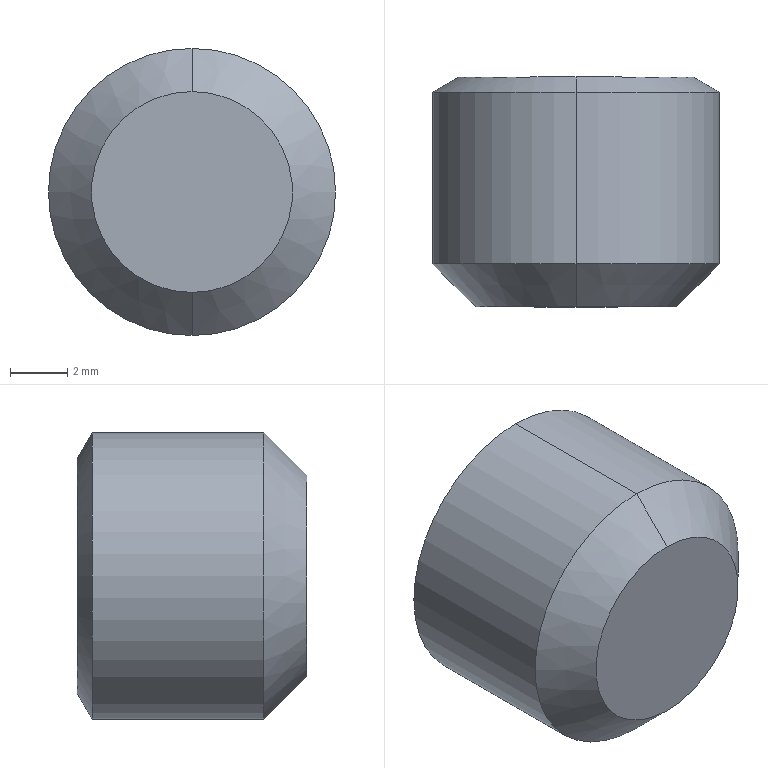Part | STEP file | 0229_Z_SCCN50-22_2 | 1 solid | 22 faces | box 10 x 8 x 10 mm | volume 459 mm3 | cone 11 | plane 9 | cylinder 2 | commonest cylinder face diameters 10 x2